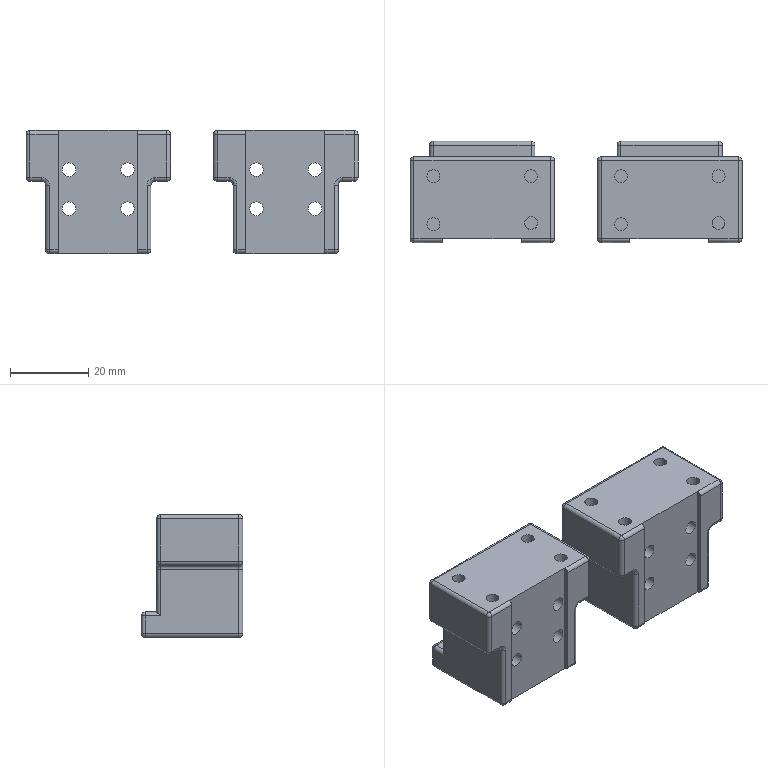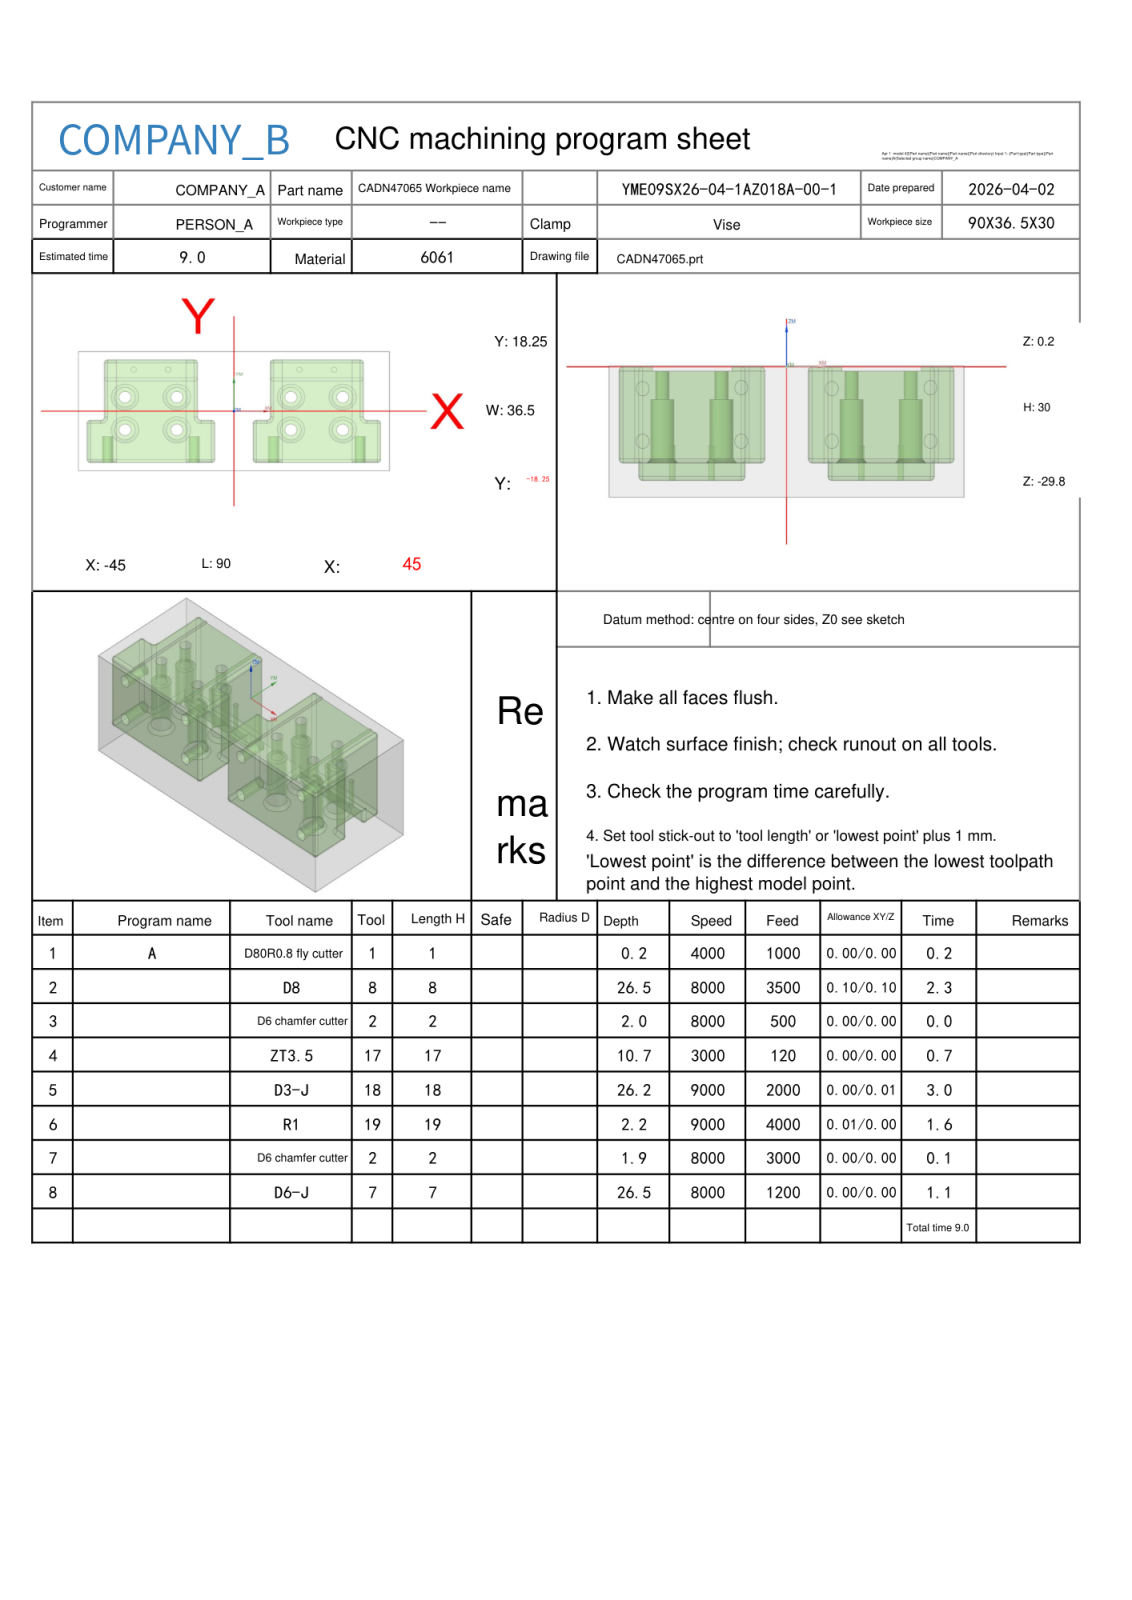NC program | NX | posted by the shop | part box 85 x 26 x 31.5 mm
Lines 34 to 963 of 17928:
N2 T08 M06
(D8  D=8. R=0. H=08 ce=0.12 di=0.10)
G00 G90 G54 X-7.417 Y27.75 M03 S8000
G43 H08 Z20.
M08
Z-11.65
G01 X-7.399 Y27.652 Z-12.275 F3500.
X-7.381 Y27.553 Z-12.522
X-7.362 Y27.455 Z-12.704
X-7.344 Y27.357 Z-12.85
X-7.326 Y27.259 Z-12.973
X-7.307 Y27.16 Z-13.078
X-7.289 Y27.062 Z-13.17
X-7.271 Y26.964 Z-13.25
X-7.253 Y26.865 Z-13.32
X-7.234 Y26.767 Z-13.382
X-7.216 Y26.669 Z-13.436
X-7.198 Y26.57 Z-13.483
X-7.179 Y26.472 Z-13.524
X-7.161 Y26.374 Z-13.558
X-7.143 Y26.275 Z-13.587
X-7.124 Y26.177 Z-13.61
X-7.106 Y26.079 Z-13.627
X-7.088 Y25.981 Z-13.64
X-7.07 Y25.882 Z-13.648
X-7.051 Y25.784 Z-13.65
X-6.735 Y24.087
G03 X-6.52 Y23.8 I.407 J.081
X-3.035 Y23.29 I3.485 J11.664
G01 X-2.959 Y23.291
G03 X5.541 Y23.197 I8.5 J383.732
X7.208 Y23.2 I0.0 J383.826
G01 X43.748 Y23.177
G02 X48.952 Y19.297 I-.2 J-5.698
X49.853 Y13.936 I-16.084 J-5.459
X49.952 Y5.979 I-320.175 J-7.957
X49.949 Y4.817 I-320.274 J0.0
G01 X49.93 Y-16.922
G02 X45.964 Y-22.245 I-5.734 J.133
X40.656 Y-23.107 I-5.396 J16.465
X32.105 Y-23.205 I-8.551 J372.4
X30.157 Y-23.2 I0.0 J372.498
G01 X-43.722 Y-23.178
G02 X-48.925 Y-19.363 I.164 J5.679
X-49.852 Y-13.943 I15.832 J5.497
X-49.951 Y-5.994 I319.545 J7.949
X-49.949 Y-4.885 I319.643 J0.0
G01 X-49.928 Y16.975
G02 X-46.124 Y22.171 I5.673 J-.162
X-41.009 Y23.087 I5.356 J-15.177
X-32.909 Y23.207 I8.101 J-272.057
X-30.871 Y23.2 I0.0 J-272.178
G01 X-8.531 Y23.18
G03 X2.726 Y22.593 I11.257 J107.591
X4.274 Y22.604 I0.0 J108.179
G01 X42.268 Y22.579
G02 X47.867 Y18.761 I-.276 J-6.42
X49.168 Y13.064 I-14.142 J-6.226
X49.372 Y3.967 I-203.381 J-9.097
X49.349 Y.947 I-203.584 J0.0
X49.374 Y-5.503 I-840.898 J-6.451
X49.311 Y-15.777 I-840.923 J0.0
X45.587 Y-21.087 I-6.372 J.508
X40.016 Y-22.405 I-6.171 J13.653
X32.491 Y-22.608 I-7.525 J139.612
X30.841 Y-22.598 I0.0 J139.815
G01 X-42.127 Y-22.584
G02 X-47.848 Y-18.801 I.132 J6.416
X-49.151 Y-13.283 I13.691 J6.147
X-49.362 Y-5.404 I147.274 J7.88
X-49.348 Y-3.388 I147.485 J0.0
G01 X-49.334 Y15.377
G02 X-45.515 Y21.116 I6.425 J-.136
X-39.818 Y22.418 I6.224 J-14.115
X-30.614 Y22.622 I9.205 J-206.95
X-27.522 Y22.599 I0.0 J-207.154
G01 X-9.802 Y22.58
G03 X-1.042 Y22.08 I24.784 J357.117
X8.9 Y22.001 I9.942 J621.459
G01 X9.308
X40.888 Y21.978
G02 X47.15 Y17.716 I-.301 J-7.173
X48.525 Y11.911 I-14.94 J-6.604
X48.77 Y3.018 I-161.204 J-8.894
X48.749 Y.396 I-161.449 J0.0
X48.768 Y-5.08 I-756.243 J-5.476
X48.711 Y-14.383 I-756.263 J0.0
X44.383 Y-20.446 I-7.164 J.538
X38.389 Y-21.798 I-6.658 J15.551
X30.593 Y-22.005 I-7.796 J146.386
X29.033 Y-21.997 I0.0 J146.594
G01 X-40.887 Y-21.977
G02 X-47.188 Y-17.637 I.307 J7.19
X-48.532 Y-11.823 I15.268 J6.591
X-48.761 Y-3.629 I146.128 J8.194
X-48.748 Y-1.628 I146.357 J0.0
X-48.774 Y4.932 I825.074 J6.56
X-48.721 Y14.232 I825.1 J0.0
X-44.466 Y20.399 I7.163 J-.39
X-38.661 Y21.774 I6.602 J-14.932
X-30.409 Y22.013 I8.252 J-142.736
X-28.346 Y21.998 I0.0 J-142.974
X-21.564 Y22.022 I6.782 J-933.536
X-9.847 Y21.949 I0.0 J-933.561
G03 X6.608 Y21.392 I16.455 J242.794
X8.709 Y21.401 I0.0 J243.351
G01 X39.508 Y21.379
G02 X46.528 Y16.624 I-.168 J-7.807
X47.925 Y10.454 I-16.532 J-6.985
X48.158 Y2.18 I-146.606 J-8.274
X48.147 Y.379 I-146.839 J0.0
X48.164 Y-4.609 I-740.488 J-4.988
X48.117 Y-12.96 I-740.505 J0.0
X43.365 Y-19.788 I-7.781 J.348
X37.31 Y-21.168 I-6.923 J16.4
X28.888 Y-21.41 I-8.422 J146.587
X26.935 Y-21.397 I0.0 J146.829
G01 X-39.505 Y-21.377
G02 X-46.581 Y-16.513 I.175 J7.834
X-47.926 Y-10.452 I16.814 J6.911
X-48.159 Y-2.082 I150.067 J8.37
X-48.147 Y-.197 I150.3 J0.0
X-48.17 Y4.817 I551.023 J5.014
X-48.108 Y13.082 I551.045 J0.0
X-43.291 Y19.816 I7.796 J-.487
X-37.171 Y21.177 I6.946 J-16.796
X-28.535 Y21.412 I8.637 J-158.428
X-26.376 Y21.398 I0.0 J-158.663
X-20.713 Y21.421 I5.663 J-676.696
X-10.277 Y21.341 I0.0 J-676.72
G03 X7.904 Y20.793 I18.18 J301.596
X10.089 Y20.801 I0.0 J302.143
G01 X38.128 Y20.783
X38.191
G02 X45.937 Y15.557 I0.0 J-8.354
X47.339 Y8.958 I-18.351 J-7.347
X47.558 Y.321 I-170.119 J-8.638
X47.547 Y-1.598 I-170.338 J0.0
X47.571 Y-5.371 I-291.361 J-3.774
X47.496 Y-11.996 I-291.385 J0.0
X46.518 Y-15.525 I-8.803 J.541
G01 X46.446 Y-16.075
X45.934 Y-17.31
X45.12 Y-18.37
X44.06 Y-19.184
G02 X42.706 Y-19.711 I-4.87 J10.505
X31.571 Y-20.776 I-11.135 J57.7
X30.866 Y-20.772 I0.0 J58.765
G01 X-37.914 Y-20.787
X-38.006 Y-20.788
G02 X-42.267 Y-19.769 I0.0 J9.42
G01 X-42.825 Y-19.696
X-44.06 Y-19.184
X-45.12 Y-18.37
X-45.934 Y-17.31
G02 X-46.469 Y-15.897 I6.036 J3.092
X-47.516 Y-5.055 I55.618 J10.842
X-47.514 Y-4.636 I56.665 J0.0
X-47.571 Y3.279 I553.028 J7.914
X-47.504 Y11.883 I553.085 J0.0
X-42.449 Y19.121 I8.266 J-.389
X-36.165 Y20.572 I7.432 J-17.854
X-27.386 Y20.809 I8.779 J-162.3
X-25.37 Y20.797 I0.0 J-162.538
X-20.357 Y20.823 I5.013 J-478.567
X-9.931 Y20.71 I0.0 J-478.593
G03 X8.982 Y20.184 I18.913 J339.794
X12.55 Y20.202 I0.0 J340.32
G01 X36.928 Y20.181
X37.081 Y20.183
G02 X42.949 Y18.001 I0.0 J-8.981
X46.119 Y12.166 I-7.774 J-8.002
X46.889 Y4.442 I-38.358 J-7.724
G01 Y4.297
G02 X46.958 Y-3.71 I-463.06 J-8.007
X46.905 Y-10.682 I-463.129 J0.0
X46.62 Y-12.705 I-17.266 J1.405
X46.643 Y-13.553 I-15.623 J-.847
X46.518 Y-15.525 I-15.646 J0.0
G03 X46.643 Y-13.553 I-15.521 J1.972
X46.62 Y-12.705 I-15.646 J0.0
X46.635 Y-9.285 I-396.595 J3.42
X46.59 Y-3.365 I-396.61 J0.0
G02 X46.345 Y5.852 I848.952 J27.256
G03 X45.342 Y12.78 I-27.393 J-.427
X41.349 Y18.165 I-8.94 J-2.457
X39.17 Y19.1 I-5.624 J-10.1
X37.825 Y19.696 I-3.393 J-5.843
G01 X36.502 Y19.87
X11.285 Y19.854
G02 X4.614 Y19.734 I-6.671 J185.252
X-6.463 Y20.065 I0.0 J185.372
G03 X-18.015 Y20.339 I-11.552 J-243.185
X-21.218 Y20.318 I0.0 J-243.459
X-24.498 Y20.336 I-3.28 J-292.432
X-34.776 Y20.156 I0.0 J-292.45
X-41.348 Y18.898 I.645 J-21.161
X-46.72 Y11.992 I3.007 J-7.882
X-47.072 Y6.111 I48.972 J-5.881
X-47.06 Y5.046 I49.324 J0.0
X-47.085 Y1.447 I260.434 J-3.599
X-46.886 Y-8.752 I260.459 J0.0
G01 X-46.62 Y-11.72
Y-14.748
X-46.464 Y-15.938
X-46.62 Y-14.748
X-46.598 Y-3.46
G03 X-46.434 Y6.038 I-275.468 J9.498
X-46.435 Y6.811 I-275.632 J0.0
G02 X-46.439 Y7.242 I23.54 J.431
X-45.866 Y12.408 I23.544 J0.0
X-40.532 Y18.207 I8.403 J-2.376
G01 X-40.099 Y18.387
X-39.06 Y19.184
X-37.825 Y19.696
X-36.5 Y19.87
X-11.498
G03 X-.21 Y19.227 I13.04 J129.492
X4.959 Y19.155 I5.169 J185.339
X8.974 Y19.198 I0.0 J185.412
G01 X10.175 Y19.696
X11.5 Y19.87
X10.175 Y19.696
G02 X6.166 Y18.76 I-4.009 J8.123
G01 X6.035 Y18.761
G02 X2.744 Y18.726 I-3.291 J152.625
X-8.909 Y19.171 I0.0 J152.661
G01 X-10.175 Y19.696
X-10.829 Y19.782
X-10.175 Y19.696
G03 X-7.724 Y18.773 I6.321 J13.079
X-.555 Y18.183 I7.335 J45.22
X2.331 Y18.107 I2.886 J55.318
X7.201 Y18.322 I0.0 J55.393
X8.065 Y18.513 I-1.852 J10.435
G01 X8.94 Y19.184
G02 X7.527 Y18.241 I-3.642 J3.93
X3.558 Y17.705 I-3.969 J14.429
X3.291 Y17.708 I0.0 J14.965
X1.22 Y17.674 I-2.071 J62.673
X-6.803 Y18.189 I0.0 J62.707
X-8.051 Y18.502 I3.799 J17.791
G01 X-8.94 Y19.184
G03 X-7.226 Y18.046 I4.596 J5.062
X-2.406 Y17.251 I5.308 J17.176
X1.138 Y17.106 I3.544 J43.161
X5.726 Y17.349 I0.0 J43.306
X7.46 Y17.837 I-.554 J5.302
G02 X8.022 Y18.48 I2.822 J-1.901
G03 X7.418 Y17.78 I2.555 J-2.814
G02 X4.827 Y16.913 I-3.018 J4.72
X.659 Y16.676 I-4.168 J36.392
X-5.812 Y17.252 I0.0 J36.63
X-7.498 Y17.874 I.781 J4.717
G01 X-7.88 Y18.37
G03 X-5.845 Y16.932 I2.782 J1.778
X.068 Y16.153 I5.912 J22.026
X.316 Y16.154 I0.0 J22.805
X1.337 Y16.128 I1.021 J20.065
X5.847 Y16.641 I0.0 J20.091
X6.989 Y17.162 I-.55 J2.717
G01 X7.468 Y17.834
X6.867 Y17.004
G02 X4.052 Y15.968 I-3.362 J4.789
X.478 Y15.713 I-3.574 J24.949
X-5.295 Y16.383 I0.0 J25.204
X-6.973 Y17.137 I1.192 J4.9
G01 X-7.431 Y17.786
G03 X-6.772 Y16.88 I15.131 J10.312
X-3.753 Y15.62 I3.966 J5.256
X.49 Y15.197 I4.243 J21.028
X4.738 Y15.621 I0.0 J21.452
X6.725 Y16.532 I-.903 J4.594
G01 X7.027 Y17.215
G02 X5.556 Y15.651 I-2.172 J.569
X.984 Y14.808 I-4.573 J11.967
X.539 Y14.815 I0.0 J12.811
X.011 Y14.807 I-.528 J16.481
X-5.325 Y15.694 I0.0 J16.49
X-6.779 Y16.616 I1.16 J3.435
G01 X-7.008 Y17.171
G03 X-5.366 Y15.403 I2.612 J.78
X-.07 Y14.321 I5.296 J12.416
G01 X.095 Y14.322
G03 X.823 Y14.301 I.728 J12.909
X5.344 Y15.118 I0.0 J12.929
X6.517 Y15.925 I-.806 J2.426
G01 X6.761 Y16.574
X6.441 Y15.758
G02 X4.024 Y14.383 I-3.327 J3.039
X.277 Y13.915 I-3.747 J14.746
X-4.823 Y14.795 I0.0 J15.215
X-6.495 Y15.885 I1.542 J4.192
G01 X-6.738 Y16.519
G03 X-6.29 Y15.517 I3.765 J1.082
X-3.3 Y13.908 I4.151 J4.133
X.297 Y13.435 I3.596 J13.429
X4.611 Y14.121 I0.0 J13.903
X6.455 Y15.404 I-1.016 J3.428
G01 X6.553 Y16.064
X6.554 Y16.012
G02 X5.609 Y14.403 I-1.843 J0.0
X1.317 Y13.122 I-4.523 J7.323
X.129 Y13.065 I-1.188 J12.238
X-4.993 Y14.182 I0.0 J12.296
X-6.466 Y15.454 I1.422 J3.137
G01 X-6.54 Y15.965
G03 X-5.51 Y14.194 I2.165 J.074
X-.777 Y12.667 I5.097 J7.704
X.443 Y12.599 I1.22 J10.859
X5.011 Y13.6 I0.0 J10.927
X6.376 Y14.771 I-1.35 J2.953
G01 X6.474 Y15.467
X6.475 Y15.421
G02 X5.45 Y13.631 I-2.077 J0.0
X.814 Y12.274 I-4.652 J7.298
X.044 Y12.247 I-.769 J10.771
X-5.026 Y13.511 I0.0 J10.799
X-6.393 Y14.85 I1.513 J2.913
G01 X-6.472 Y15.445
G03 X-5.296 Y13.366 I2.483 J.032
X-.197 Y11.82 I5.126 J7.721
X.518 Y11.793 I.715 J9.521
X5.213 Y13.027 I0.0 J9.548
X6.371 Y14.233 I-1.376 J2.481
G01 X6.38 Y14.752
G02 X6.395 Y14.531 I-1.644 J-.221
X5.771 Y13.235 I-1.658 J0.0
X1.794 Y11.563 I-4.604 J5.388
X.16 Y11.436 I-1.634 J10.42
X-4.808 Y12.679 I0.0 J10.547
X-6.371 Y14.266 I1.691 J3.23
G01 X-6.38 Y14.748
X-6.387 Y14.579
G03 X-5.544 Y12.887 I2.12 J0.0
X-.978 Y11.081 I5.11 J6.243
X.331 Y10.993 I1.31 J9.643
X4.956 Y12.162 I0.0 J9.731
X6.375 Y13.622 I-1.427 J2.807
G01 X6.38 Y14.254
G02 X6.399 Y13.982 I-1.996 J-.272
X5.559 Y12.346 I-2.014 J0.0
X1.017 Y10.697 I-4.788 J6.109
X.069 Y10.65 I-.948 J9.626
X-4.975 Y12.069 I0.0 J9.672
X-6.38 Y13.688 I1.659 J2.86
G01 Y14.288
G03 X-6.398 Y13.995 I2.347 J-.293
X-5.478 Y12.123 I2.365 J0.0
X-.651 Y10.267 I5.18 J6.266
X.362 Y10.21 I1.013 J9.059
X5.152 Y11.57 I0.0 J9.116
X6.38 Y12.978 I-1.441 J2.497
G01 Y13.638
G02 X6.402 Y13.335 I-2.136 J-.304
X5.496 Y11.578 I-2.157 J0.0
X.636 Y9.896 I-4.886 J6.258
X-.003 Y9.874 I-.639 J9.051
X-5.177 Y11.494 I0.0 J9.074
X-6.38 Y13.013 I1.814 J2.672
G01 Y13.673
G03 X-6.401 Y13.347 I2.524 J-.325
X-5.371 Y11.302 I2.545 J0.0
X-.134 Y9.46 I5.236 J6.518
G01 X-.105
G03 X.439 Y9.442 I.544 J8.535
X5.363 Y11.002 I0.0 J8.553
X6.38 Y12.271 I-1.523 J2.263
G01 Y12.931
G02 X6.405 Y12.61 I-2.092 J-.321
X5.597 Y10.946 I-2.117 J0.0
X.946 Y9.143 I-4.92 J5.789
X.045 Y9.098 I-.902 J8.996
X-5.12 Y10.718 I0.0 J9.041
X-6.38 Y12.303 I1.953 J2.845
G01 Y12.903
G03 X-6.396 Y12.619 I2.545 J-.284
X-5.384 Y10.58 I2.561 J0.0
X-.129 Y8.69 I5.255 J6.36
G01 X-.105
G03 X.43 Y8.673 I.535 J8.373
X5.45 Y10.341 I0.0 J8.39
X6.38 Y11.549 I-1.57 J2.17
G01 Y12.269
G02 X6.405 Y11.933 I-2.283 J-.336
X6.2 Y10.982 I-2.307 J0.0
X3.297 Y8.86 I-4.358 J2.915
X.171 Y8.323 I-3.126 J8.823
X-4.927 Y9.833 I0.0 J9.361
X-6.38 Y11.573 I1.951 J3.105
G01 Y12.233
G03 X-6.4 Y11.908 I2.591 J-.325
X-5.403 Y9.855 I2.611 J0.0
X-.106 Y7.92 I5.297 J6.284
G01 X.028 Y7.922
G03 X.423 Y7.912 I.395 J8.325
X5.415 Y9.573 I0.0 J8.334
X6.38 Y10.819 I-1.613 J2.246
G01 Y11.539
G02 X6.405 Y11.203 I-2.305 J-.336
X6.202 Y10.252 I-2.329 J0.0
X3.286 Y8.101 I-4.395 J2.907
X.165 Y7.561 I-3.121 J8.749
X-4.876 Y9.048 I0.0 J9.289
X-6.38 Y10.844 I2. J3.203
G01 Y11.564
G03 X-6.404 Y11.204 I2.672 J-.36
X-5.396 Y9.102 I2.696 J0.0
X-.098 Y7.156 I5.298 J6.241
G01 X.072 Y7.158
G03 X.442 Y7.15 I.37 J8.151
X5.549 Y8.945 I0.0 J8.159
X6.38 Y10.081 I-1.632 J2.066
G01 Y10.801
G02 X6.404 Y10.465 I-2.33 J-.337
X6.206 Y9.52 I-2.354 J0.0
X3.317 Y7.357 I-4.406 J2.876
X.161 Y6.801 I-3.156 J8.673
X-4.872 Y8.293 I0.0 J9.23
X-6.38 Y10.1 I2.026 J3.225
G01 Y10.76
G03 X-6.399 Y10.438 I2.673 J-.322
X-5.361 Y8.314 I2.692 J0.0
X-.053 Y6.39 I5.308 J6.361
X.295 Y6.398 I0.0 J8.285
G01 X.474 Y6.396
G03 X5.589 Y8.235 I0.0 J8.031
X6.38 Y9.344 I-1.611 J1.985
G01 Y10.064
G02 X6.405 Y9.727 I-2.294 J-.337
X5.518 Y7.903 I-2.319 J0.0
X.47 Y6.064 I-5.048 J6.009
G01 X.395
G02 X-.046 Y6.053 I-.441 J8.465
X-5.33 Y7.901 I0.0 J8.476
X-6.38 Y9.346 I2.171 J2.682
G01 Y10.006
G03 X-6.401 Y9.676 I2.627 J-.33
X-5.418 Y7.617 I2.647 J0.0
X-.095 Y5.635 I5.323 J6.158
X.114 Y5.638 I0.0 J8.14
X.433 Y5.632 I.319 J8.096
X5.57 Y7.468 I0.0 J8.102
X6.38 Y8.593 I-1.665 J2.053
G01 Y9.313
G02 X6.404 Y8.977 I-2.335 J-.337
X6.202 Y8.02 I-2.359 J0.0
X3.307 Y5.844 I-4.438 J2.89
X.151 Y5.278 I-3.155 J8.525
X-5.003 Y6.881 I0.0 J9.09
X-6.38 Y8.599 I2.088 J3.085
G01 Y9.259
G03 X-6.399 Y8.937 I2.688 J-.322
X-5.363 Y6.807 I2.707 J0.0
X-.045 Y4.871 I5.318 J6.333
X.382 Y4.882 I0.0 J8.27
G01 X.468 Y4.881
G03 X5.568 Y6.716 I0.0 J8.005
X6.38 Y7.849 I-1.664 J2.05
G01 Y8.569
G02 X6.405 Y8.231 I-2.3 J-.337
X5.541 Y6.423 I-2.325 J0.0
X.48 Y4.55 I-5.065 J5.914
X-.058 Y4.533 I-.538 J8.363
X-5.431 Y6.483 I0.0 J8.38
X-6.38 Y7.841 I2.215 J2.559
G01 Y8.501
G03 X-6.398 Y8.186 I2.705 J-.315
X-5.346 Y6.035 I2.723 J0.0
X-.032 Y4.111 I5.314 J6.378
X.47 Y4.126 I0.0 J8.302
G01 X.491
G03 X5.627 Y6.019 I0.0 J7.915
X6.38 Y7.101 I-1.668 J1.964
G01 Y7.821
G02 X6.405 Y7.483 I-2.318 J-.338
X5.511 Y5.642 I-2.342 J0.0
X.449 Y3.791 I-5.062 J5.992
G01 X.39
G02 X-.068 Y3.778 I-.458 J8.35
X-5.418 Y5.713 I0.0 J8.362
X-6.38 Y7.09 I2.174 J2.545
G01 Y7.75
G03 X-6.4 Y7.426 I2.687 J-.325
X-5.378 Y5.307 I2.706 J0.0
X-.06 Y3.357 I5.317 J6.271
X.334 Y3.366 I0.0 J8.222
G01 X.454 Y3.365
G03 X5.582 Y5.223 I0.0 J8.005
X6.38 Y6.342 I-1.714 J2.067
G01 Y7.062
G02 X6.405 Y6.725 I-2.301 J-.337
X5.539 Y4.915 I-2.326 J0.0
X.478 Y3.036 I-5.073 J5.911
X-.05 Y3.02 I-.528 J8.404
X-5.37 Y4.913 I0.0 J8.421
X-6.38 Y6.335 I2.147 J2.594
G01 Y6.995
G03 X-6.399 Y6.673 I2.704 J-.322
X-5.358 Y4.532 I2.723 J0.0
X-.041 Y2.597 I5.317 J6.337
X.468 Y2.612 I0.0 J8.272
G01 X.484
G03 X5.629 Y4.513 I0.0 J7.914
X6.38 Y5.595 I-1.663 J1.956
G01 Y6.315
G02 X6.405 Y5.977 I-2.308 J-.338
X5.566 Y4.186 I-2.332 J0.0
X.521 Y2.281 I-5.088 J5.842
X-.051 Y2.261 I-.572 J8.387
X-5.392 Y4.176 I0.0 J8.406
X-6.38 Y5.575 I2.185 J2.592
G01 Y6.235
G03 X-6.401 Y5.899 I2.632 J-.336
X-5.435 Y3.851 I2.654 J0.0
X-.12 Y1.851 I5.315 J6.06
G01 X.02 Y1.852
G03 X.383 Y1.844 I.363 J8.182
X5.493 Y3.634 I0.0 J8.19
X6.38 Y4.839 I-1.696 J2.176
G01 Y5.559
G02 X6.405 Y5.221 I-2.313 J-.338
X5.537 Y3.403 I-2.338 J0.0
X.438 Y1.518 I-5.098 J5.951
G01 X.345 Y1.519
G02 X-.093 Y1.507 I-.437 J8.255
X-5.495 Y3.517 I0.0 J8.267
X-6.38 Y4.819 I2.198 J2.445
G01 Y5.479
G03 X-6.399 Y5.158 I2.7 J-.321
X-5.36 Y3.021 I2.719 J0.0
X-.056 Y1.085 I5.305 J6.3
X.378 Y1.096 I0.0 J8.236
G01 X.473
G03 X5.662 Y3.036 I0.0 J7.91
X6.38 Y4.077 I-1.669 J1.919
G01 Y4.797
G02 X6.404 Y4.46 I-2.311 J-.337
X5.509 Y2.622 I-2.335 J0.0
X.415 Y.759 I-5.093 J6.03
G01 X.256 Y.76
G02 X-.095 Y.753 I-.351 J8.282
X-5.431 Y2.698 I0.0 J8.289
X-6.38 Y4.059 I2.229 J2.567
G01 Y4.719
G03 X-6.398 Y4.403 I2.709 J-.316
X-5.35 Y2.253 I2.728 J0.0
X-.011 Y.323 I5.339 J6.42
X.647 Y.349 I0.0 J8.35
X5.707 Y2.326 I-.115 J7.759
X6.38 Y3.326 I-1.712 J1.879
G01 Y4.046
G02 X6.404 Y3.708 I-2.357 J-.338
X6.205 Y2.754 I-2.381 J0.0
X3.336 Y.565 I-4.454 J2.862
X.138 Y-.017 I-3.197 J8.494
X-4.957 Y1.548 I0.0 J9.076
X-6.38 Y3.307 I2.078 J3.136
G01 Y3.967
G03 X-6.401 Y3.636 I2.657 J-.332
X-5.418 Y1.563 I2.677 J0.0
X-4.791 Y1.076 I3.291 J3.591
X-1.926 Y-.159 I6.745 J11.699
X.195 Y-.411 I2.121 J8.811
X3.176 Y.093 I0.0 J9.063
G01 X3.667 Y.515
G03 X5.736 Y1.712 I-3.34 J8.16
X6.38 Y2.641 I-1.313 J1.599
G01 Y3.301
G02 X6.404 Y2.987 I-2.016 J-.314
X5.347 Y1.199 I-2.04 J0.0
G01 X4.791 Y1.076
G03 X6.37 Y2.09 I-.105 J1.901
G01 X6.38 Y2.634
G02 X6.403 Y2.392 I-1.256 J-.242
X5.781 Y1.295 I-1.279 J0.0
G01 X5.371 Y1.204
G03 X6.35 Y1.754 I-.033 J1.206
G01 X6.38 Y2.152
X6.397 Y1.993
G02 X6.15 Y1.435 I-.755 J0.0
X5.887 Y1.349 I-.263 J.358
X5.443 Y1.793 I0.0 J.444
X5.598 Y2.13 I.444 J0.0
X5.936 Y2.289 I.338 J-.282
X6.376 Y1.849 I0.0 J-.44
G01 X6.369 Y1.768
G02 X5.796 Y1.297 I-.573 J.113
G01 X5.789
G03 X3.084 Y.016 I.609 J-4.783
G02 X.146 Y-.735 I-2.938 J5.378
X-.552 Y-.695 I0.0 J6.128
X-2.854 Y-.183 I.491 J7.643
G01 X-3.667 Y.514
G03 X-2.1 Y-.65 I4.48 J4.391
X.188 Y-1.086 I2.288 J5.783
X2.425 Y-.67 I0.0 J6.219
G02 X3.168 Y.087 I3.265 J-2.464
G03 X2.435 Y-.687 I1.599 J-2.251
G02 X.11 Y-1.36 I-2.325 J3.676
X-.505 Y-1.317 I0.0 J4.349
X-2.412 Y-.73 I.092 J3.69
G01 X-2.713 Y-.304
G03 X-.692 Y-1.576 I2.247 J1.33
X.171 Y-1.665 I.864 J4.125
X2.049 Y-1.224 I0.0 J4.215
G01 X2.479 Y-.635
G02 X.572 Y-1.839 I-1.983 J1.027
X-.042 Y-1.892 I-.614 J3.523
X-2.006 Y-1.305 I0.0 J3.576
G01 X-2.387 Y-.766
G03 X-.116 Y-2.136 I2.271 J1.198
G01 X-.078 Y-2.135
G03 X.258 Y-2.156 I.336 J2.686
X1.845 Y-1.642 I0.0 J2.707
G01 X2.092 Y-1.184
X1.85 Y-1.667
G02 X.055 Y-2.356 I-1.795 J1.995
X-.56 Y-2.285 I0.0 J2.683
X-1.876 Y-1.619 I.156 J1.941
G01 X-1.988 Y-1.331
G03 X-.632 Y-2.479 I1.585 J.496
X.107 Y-2.584 I.739 J2.568
X1.668 Y-2.08 I0.0 J2.672
G01 X1.891 Y-1.581
G02 X.738 Y-2.652 I-1.359 J.307
X.001 Y-2.767 I-.737 J2.305
X-1.696 Y-2.072 I0.0 J2.42
G01 X-1.861 Y-1.659
G03 X-.311 Y-2.927 I1.653 J.439
X.128 Y-2.972 I.439 J2.144
X1.536 Y-2.459 I0.0 J2.189
G01 X1.728 Y-2.001
G02 X.551 Y-3.058 I-1.325 J.293
X-.018 Y-3.137 I-.569 J2.01
X-1.546 Y-2.471 I0.0 J2.089
G01 X-1.698 Y-2.08
G03 X-.164 Y-3.297 I1.564 J.396
X.143 Y-3.322 I.307 J1.821
X1.466 Y-2.764 I0.0 J1.846
G01 X1.556 Y-2.447
G02 X.738 Y-3.331 I-1.024 J.127
X.015 Y-3.47 I-.723 J1.81
X-1.476 Y-2.776 I0.0 J1.949
G01 X-1.534 Y-2.503
G03 X-.764 Y-3.459 I1.089 J.088
X.064 Y-3.655 I.828 J1.653
X1.442 Y-3.038 I0.0 J1.848
G01 X1.519 Y-2.622
X1.52 Y-2.641
G02 X.721 Y-3.645 I-1.03 J0.0
X.018 Y-3.785 I-.703 J1.697
X-1.448 Y-3.055 I0.0 J1.837
G01 X-1.513 Y-2.672
G03 X-.451 Y-3.874 I1.246 J.03
X.084 Y-3.96 I.535 J1.617
X1.412 Y-3.324 I0.0 J1.703
G01 X1.481 Y-2.931
Y-2.945
G02 X.678 Y-3.957 I-1.039 J0.0
X.015 Y-4.087 I-.663 J1.626
X-1.416 Y-3.347 I0.0 J1.756
G01 X-1.476 Y-2.977
G03 X-.4 Y-4.182 I1.236 J.021
X.081 Y-4.253 I.48 J1.595
X1.37 Y-3.641 I0.0 J1.666
G01 X1.45 Y-3.18
X1.451 Y-3.209
G02 X.469 Y-4.312 I-1.111 J0.0
X0.0 Y-4.379 I-.469 J1.602
X-1.379 Y-3.65 I0.0 J1.67
G01 X-1.438 Y-3.281
G03 X-.355 Y-4.482 I1.227 J.017
X.097 Y-4.55 I.452 J1.468
X1.351 Y-3.901 I0.0 J1.536
G01 X1.402 Y-3.57
Y-3.581
G02 X.65 Y-4.539 I-.986 J0.0
X.011 Y-4.669 I-.639 J1.505
X-1.356 Y-3.931 I0.0 J1.635
G01 X-1.395 Y-3.632
Y-3.64
G03 X-.544 Y-4.707 I1.095 J0.0
X.059 Y-4.825 I.604 J1.489
X1.339 Y-4.189 I0.0 J1.606
G01 X1.38 Y-3.748
X1.389 Y-3.879
G02 X.653 Y-4.815 I-.964 J0.0
X.017 Y-4.946 I-.636 J1.484
X-1.356 Y-4.18 I0.0 J1.614
G01 X-1.38 Y-3.83
X-1.385 Y-3.931
G03 X-.556 Y-4.98 I1.077 J0.0
X.063 Y-5.108 I.618 J1.424
X1.355 Y-4.417 I0.0 J1.553
G01 X1.38 Y-3.996
X1.392 Y-4.148
G02 X.696 Y-5.072 I-.961 J0.0
X.012 Y-5.229 I-.684 J1.411
X-1.367 Y-4.409 I0.0 J1.568
G01 X-1.38 Y-4.095
X-1.385 Y-4.201
G03 X-.571 Y-5.249 I1.082 J0.0
X.057 Y-5.379 I.628 J1.45
X1.346 Y-4.712 I0.0 J1.58
G01 X1.38 Y-4.334
X1.385 Y-4.429
G02 X.659 Y-5.361 I-.961 J0.0
X.007 Y-5.504 I-.652 J1.414
X-1.368 Y-4.677 I0.0 J1.557
G01 X-1.38 Y-4.367
X-1.385 Y-4.471
G03 X-.552 Y-5.53 I1.09 J0.0
X.064 Y-5.659 I.615 J1.408
X1.358 Y-4.951 I0.0 J1.537
G01 X1.38 Y-4.546
X1.39 Y-4.687
G02 X.657 Y-5.635 I-.98 J0.0
X.017 Y-5.768 I-.64 J1.474
X-1.354 Y-4.999 I0.0 J1.607
G01 X-1.38 Y-4.637
X-1.385 Y-4.745
G03 X-.569 Y-5.798 I1.087 J0.0
X.054 Y-5.925 I.623 J1.464
X1.344 Y-5.264 I0.0 J1.591
G01 X1.38 Y-4.822
X1.391 Y-4.964
G02 X.676 Y-5.901 I-.972 J0.0
X.016 Y-6.045 I-.661 J1.451
X-1.36 Y-5.257 I0.0 J1.595
G01 X-1.38 Y-4.919
X-1.385 Y-5.023
G03 X-.57 Y-6.072 I1.083 J0.0
X.055 Y-6.203 I.626 J1.433
X1.354 Y-5.511 I0.0 J1.563
G01 X1.38 Y-5.087
X1.392 Y-5.239
G02 X.693 Y-6.168 I-.967 J0.0
X.01 Y-6.325 I-.682 J1.41
X-1.367 Y-5.504 I0.0 J1.566
G01 X-1.38 Y-5.19
X-1.385 Y-5.297
G03 X-.571 Y-6.346 I1.083 J0.0
X.066 Y-6.485 I.637 J1.389
X1.36 Y-5.77 I0.0 J1.528
G01 X1.38 Y-5.432
X1.385 Y-5.524
G02 X.662 Y-6.457 I-.965 J0.0
X.007 Y-6.602 I-.655 J1.407
X-1.369 Y-5.769 I0.0 J1.552
G01 X-1.38 Y-5.462
X-1.385 Y-5.57
G03 X-.569 Y-6.621 I1.086 J0.0
X.053 Y-6.748 I.622 J1.468
X1.343 Y-6.09 I0.0 J1.595
G01 X1.38 Y-5.645
X1.39 Y-5.785
G02 X.664 Y-6.729 I-.976 J0.0
X.009 Y-6.873 I-.655 J1.418
X-1.367 Y-6.051 I0.0 J1.562
G01 X-1.38 Y-5.738
X-1.385 Y-5.84
G03 X-.535 Y-6.908 I1.096 J0.0
X.069 Y-7.033 I.604 J1.389
X1.362 Y-6.307 I0.0 J1.514
G01 X1.38 Y-5.916
X1.391 Y-6.058
G02 X.673 Y-6.999 I-.975 J0.0
X.012 Y-7.145 I-.661 J1.427
X-1.366 Y-6.331 I0.0 J1.573
G01 X-1.38 Y-6.013
X-1.385 Y-6.118
G03 X-.57 Y-7.168 I1.085 J0.0
X.053 Y-7.295 I.623 J1.469
X1.343 Y-6.638 I0.0 J1.596
G01 X1.38 Y-6.193
X1.39 Y-6.333
G02 X.657 Y-7.279 I-.977 J0.0
X.007 Y-7.421 I-.65 J1.415
X-1.368 Y-6.596 I0.0 J1.557
G01 X-1.38 Y-6.285
X-1.385 Y-6.389
G03 X-.552 Y-7.449 I1.091 J0.0
X.057 Y-7.572 I.609 J1.44
X1.353 Y-6.884 I0.0 J1.563
G01 X1.38 Y-6.459
X1.392 Y-6.61
G02 X.693 Y-7.539 I-.967 J0.0
X.014 Y-7.693 I-.679 J1.419
X-1.366 Y-6.876 I0.0 J1.573
G01 X-1.38 Y-6.56
X-1.385 Y-6.664
G03 X-.57 Y-7.716 I1.086 J0.0
X.055 Y-7.845 I.625 J1.451
X1.346 Y-7.176 I0.0 J1.58
G01 X1.38 Y-6.798
X1.385 Y-6.895
G02 X.674 Y-7.821 I-.958 J0.0
X.016 Y-7.963 I-.658 J1.452
X-1.36 Y-7.175 I0.0 J1.594
G01 X-1.38 Y-6.837
X-1.385 Y-6.942
G03 X-.57 Y-7.991 I1.083 J0.0
X.054 Y-8.12 I.625 J1.449
X1.349 Y-7.443 I0.0 J1.577
G01 X1.38 Y-7.011
X1.391 Y-7.158
G02 X.675 Y-8.094 I-.97 J0.0
X.013 Y-8.24 I-.662 J1.438
X-1.363 Y-7.439 I0.0 J1.583
G01 X-1.38 Y-7.113
X-1.385 Y-7.214
G03 X-.553 Y-8.272 I1.088 J0.0
X.062 Y-8.4 I.615 J1.413
X1.357 Y-7.694 I0.0 J1.541
G01 X1.38 Y-7.347
X1.385 Y-7.446
G02 X.692 Y-8.362 I-.951 J0.0
X.013 Y-8.515 I-.678 J1.423
X-1.365 Y-7.703 I0.0 J1.576
G01 X-1.38 Y-7.384
X-1.385 Y-7.488
G03 X-.571 Y-8.539 I1.085 J0.0
X.055 Y-8.668 I.625 J1.445
X1.35 Y-7.99 I0.0 J1.575
G01 X1.38 Y-7.559
X1.391 Y-7.704
G02 X.658 Y-8.649 I-.976 J0.0
X.008 Y-8.791 I-.65 J1.42
X-1.367 Y-7.969 I0.0 J1.561
G01 X-1.38 Y-7.656
X-1.385 Y-7.76
G03 X-.552 Y-8.82 I1.091 J0.0
X.055 Y-8.941 I.607 J1.463
X1.347 Y-8.274 I0.0 J1.584
G01 X1.38 Y-7.897
X1.384 Y-7.988
G02 X.645 Y-8.93 I-.97 J0.0
X.005 Y-9.069 I-.64 J1.409
X-1.369 Y-8.233 I0.0 J1.548
G01 X-1.38 Y-7.927
X-1.385 Y-8.035
G03 X-.569 Y-9.088 I1.087 J0.0
X.055 Y-9.216 I.624 J1.445
X1.35 Y-8.537 I0.0 J1.574
G01 X1.38 Y-8.107
X1.391 Y-8.251
G02 X.661 Y-9.198 I-.98 J0.0
X.01 Y-9.341 I-.651 J1.42
X-1.367 Y-8.515 I0.0 J1.562
G01 X-1.38 Y-8.203
X-1.385 Y-8.307
G03 X-.551 Y-9.368 I1.092 J0.0
X.057 Y-9.491 I.608 J1.45
X1.35 Y-8.813 I0.0 J1.572
G01 X1.38 Y-8.443
X1.386 Y-8.545
G02 X.675 Y-9.466 I-.953 J0.0
X.013 Y-9.612 I-.662 J1.427
X-1.366 Y-8.796 I0.0 J1.573
G01 X-1.38 Y-8.479
X-1.385 Y-8.583
G03 X-.569 Y-9.636 I1.087 J0.0
X.055 Y-9.763 I.624 J1.462
X1.346 Y-9.101 I0.0 J1.589
G01 X1.38 Y-8.722
X1.385 Y-8.818
G02 X.676 Y-9.74 I-.954 J0.0
X.009 Y-9.89 I-.667 J1.409
X-1.368 Y-9.061 I0.0 J1.559
G01 X-1.38 Y-8.751
X-1.385 Y-8.857
G03 X-.569 Y-9.91 I1.087 J0.0
X.057 Y-10.041 I.626 J1.431
X1.354 Y-9.349 I0.0 J1.562
G01 X1.38 Y-8.926
X1.392 Y-9.078
G02 X.693 Y-10.007 I-.966 J0.0
X.013 Y-10.162 I-.68 J1.415
X-1.366 Y-9.342 I0.0 J1.57
G01 X-1.38 Y-9.027
X-1.385 Y-9.132
G03 X-.564 Y-10.186 I1.088 J0.0
X.055 Y-10.311 I.618 J1.463
X1.345 Y-9.649 I0.0 J1.589
G01 X1.38 Y-9.269
X1.385 Y-9.361
G02 X.663 Y-10.295 I-.965 J0.0
X.009 Y-10.439 I-.654 J1.412
X-1.369 Y-9.607 I0.0 J1.556
G01 X-1.38 Y-9.299
X-1.385 Y-9.406
G03 X-.569 Y-10.459 I1.087 J0.0
X.053 Y-10.585 I.622 J1.469
X1.343 Y-9.929 I0.0 J1.595
G01 X1.38 Y-9.484
X1.39 Y-9.623
G02 X.658 Y-10.569 I-.978 J0.0
X.009 Y-10.71 I-.649 J1.423
X-1.367 Y-9.889 I0.0 J1.564
G01 X-1.38 Y-9.575
X-1.385 Y-9.678
G03 X-.551 Y-10.739 I1.092 J0.0
X.054 Y-10.859 I.605 J1.471
X1.342 Y-10.202 I0.0 J1.59
G01 X1.38 Y-9.754
X1.387 Y-9.876
G02 X.544 Y-10.885 I-1.026 J0.0
X.005 Y-10.981 I-.539 J1.466
X-1.365 Y-10.169 I0.0 J1.562
G01 X-1.38 Y-9.851
X-1.385 Y-9.955
G03 X-.57 Y-11.006 I1.086 J0.0
X.053 Y-11.133 I.623 J1.468
X1.342 Y-10.477 I0.0 J1.595
G01 X1.38 Y-10.03
X1.39 Y-10.169
G02 X.661 Y-11.117 I-.981 J0.0
X.01 Y-11.26 I-.651 J1.42
X-1.368 Y-10.434 I0.0 J1.562
G01 X-1.38 Y-10.123
X-1.385 Y-10.226
G03 X-.551 Y-11.287 I1.092 J0.0
X.056 Y-11.409 I.608 J1.451
X1.35 Y-10.732 I0.0 J1.573
G01 X1.38 Y-10.301
X1.391 Y-10.449
G02 X.675 Y-11.385 I-.971 J0.0
X.013 Y-11.531 I-.662 J1.427
X-1.366 Y-10.715 I0.0 J1.573